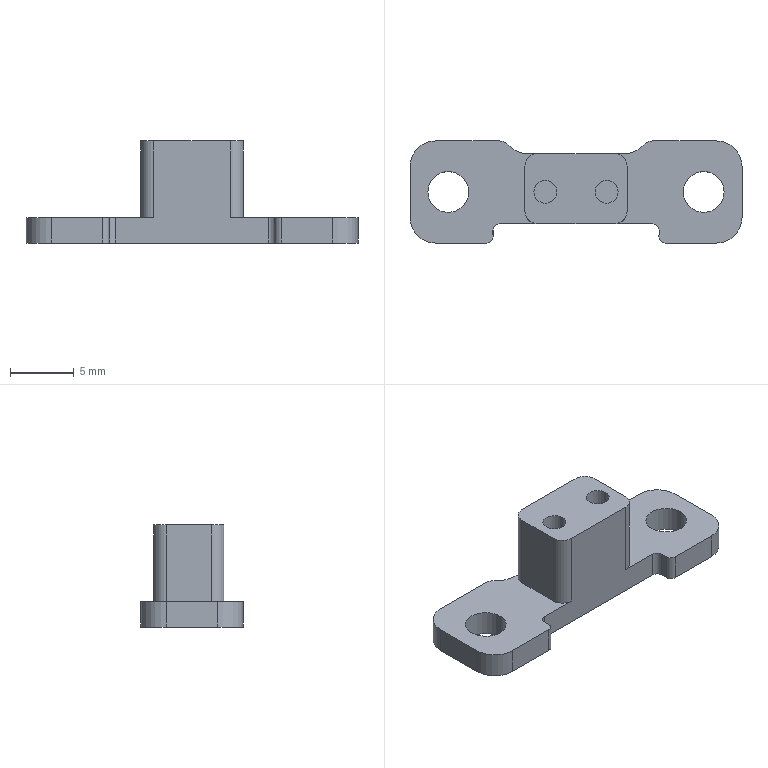NC program | Mastercam | posted with a generic post
Lines 28 to 1213 of 12913:
(8 FEM |TOOL - 8|DIA. OFF. - 8|LEN. - 8|TOOL DIA. - 8.)
N134 T8 M6
N136 G0 G54 G90 X-18.469 Y-15.865 C0. B0. S7000 M3
N138 G43 H8 Z50.
N140 Z-6.696
N142 G1 Z-7.196 F600.
N144 X-18.67 Y-15.925 Z-7.233 F4000.
N146 X-18.876 Y-15.963 Z-7.27
N148 X-19.085 Y-15.979 Z-7.307
N150 X-19.294 Y-15.973 Z-7.344
N152 X-19.501 Y-15.946 Z-7.381
N154 X-19.705 Y-15.897 Z-7.418
N156 X-19.902 Y-15.827 Z-7.455
N158 X-20.091 Y-15.736 Z-7.491
N160 X-20.269 Y-15.627 Z-7.528
N162 X-20.435 Y-15.499 Z-7.565
N164 X-20.587 Y-15.355 Z-7.602
N166 X-20.723 Y-15.196 Z-7.639
N168 X-20.841 Y-15.023 Z-7.676
N170 X-20.941 Y-14.839 Z-7.713
N172 X-21.021 Y-14.646 Z-7.75
N174 X-21.829 Y-12.359
N176 X-22.16 Y-11.421 Z-7.849
N178 X-22.398 Y-10.746 Z-7.92
N180 X-22.476 Y-10.561 Z-7.94
N182 X-22.573 Y-10.386 Z-7.96
N184 X-22.689 Y-10.222 Z-7.98
N186 X-22.823 Y-10.073 Z-8.
N188 X-23.064 Y-9.697
N190 X-23.25 Y-9.308
N192 X-23.4 Y-8.939
N194 X-23.521 Y-8.596
N196 X-23.614 Y-8.279
N198 X-23.685 Y-7.988
N200 X-23.738 Y-7.719
N202 X-23.777 Y-7.471
N204 X-23.83 Y-7.036
N206 X-23.862 Y-6.643
N208 X-23.882 Y-6.282
N210 X-23.893 Y-5.944
N212 X-23.9 Y-5.621
N214 X-23.904 Y-5.309
N216 X-23.906 Y-5.005
N218 X-23.907 Y-4.706
N220 Y-4.41
N222 X-23.906 Y-4.117
N224 X-23.905 Y-3.825
N226 X-23.904 Y-3.535
N228 X-23.903 Y-3.244
N230 X-23.901 Y-2.954
N232 X-23.9 Y-2.664
N234 X-23.898 Y-2.374
N236 X-23.897 Y-2.084
N238 X-23.895 Y-1.794
N240 X-23.894 Y-1.504
N242 X-23.892 Y-1.214
N244 X-23.891 Y-.924
N246 X-23.889 Y-.634
N248 X-23.887 Y-.344
N250 X-23.886 Y-.053
N252 X-23.884 Y.237
N254 X-23.883 Y.527
N256 X-23.881 Y.817
N258 X-23.88 Y1.108
N260 X-23.878 Y1.398
N262 X-23.877 Y1.688
N264 X-23.875 Y1.979
N266 X-23.874 Y2.269
N268 X-23.872 Y2.56
N270 X-23.871 Y2.85
N272 X-23.869 Y3.141
N274 X-23.867 Y3.432
N276 X-23.866 Y3.722
N278 X-23.864 Y4.013
N280 X-23.863 Y4.304
N282 X-23.861 Y4.595
N284 X-23.86 Y4.885
N286 X-23.858 Y5.176
N288 X-23.857 Y5.467
N290 X-23.855 Y5.758
N292 X-23.854 Y6.049
N294 X-23.852 Y6.34
N296 X-23.851 Y6.631
N298 X-23.832 Y7.022
N300 X-23.763 Y7.461
N302 X-23.646 Y7.891
N304 X-23.483 Y8.306
N306 X-23.28 Y8.696
N308 X-23.046 Y9.056
N310 X-22.786 Y9.384
N312 X-22.508 Y9.678
N314 X-22.22 Y9.938
N316 X-21.926 Y10.165
N318 X-21.631 Y10.362
N320 X-21.34 Y10.531
N322 X-21.054 Y10.677
N324 X-20.776 Y10.801
N326 X-20.507 Y10.906
N328 X-20.246 Y10.996
N330 X-19.995 Y11.072
N332 X-19.754 Y11.137
N334 X-19.521 Y11.191
N336 X-19.09 Y11.276
N338 X-18.683 Y11.339
N340 X-18.298 Y11.386
N342 X-17.931 Y11.421
N344 X-17.579 Y11.447
N346 X-17.239 Y11.466
N348 X-16.909 Y11.481
N350 X-16.588 Y11.492
N352 X-16.272 Y11.5
N354 X-15.962 Y11.505
N356 X-15.655 Y11.509
N358 X-15.352 Y11.512
N360 X-15.051 Y11.513
N362 X-14.753 Y11.514
N364 X-14.456
N366 X-14.16
N368 X-13.865
N370 X-13.571 Y11.513
N372 X-13.278 Y11.512
N374 X-12.985 Y11.51
N376 X-12.692 Y11.509
N378 X-12.399 Y11.508
N380 X-12.106 Y11.506
N382 X-11.814 Y11.505
N384 X-11.521 Y11.504
N386 X-11.229 Y11.502
N388 X-10.936 Y11.501
N390 X-10.644 Y11.499
N392 X-10.352 Y11.497
N394 X-10.059 Y11.496
N396 X-9.767 Y11.494
N398 X-9.475 Y11.493
N400 X-9.182 Y11.491
N402 X-8.89 Y11.49
N404 X-8.597 Y11.488
N406 X-8.305 Y11.487
N408 X-8.012 Y11.485
N410 X-7.72 Y11.484
N412 X-7.428 Y11.482
N414 X-7.135 Y11.48
N416 X-6.843 Y11.479
N418 X-6.55 Y11.477
N420 X-6.258 Y11.476
N422 X-5.965 Y11.474
N424 X-5.672 Y11.473
N426 X-5.38 Y11.471
N428 X-5.087 Y11.47
N430 X-4.795 Y11.468
N432 X-4.502 Y11.467
N434 X-4.21 Y11.465
N436 X-3.917 Y11.463
N438 X-3.624 Y11.462
N440 X-3.332 Y11.46
N442 X-3.039 Y11.459
N444 X-2.747 Y11.457
N446 X-2.454 Y11.456
N448 X-2.161 Y11.454
N450 X-1.869 Y11.453
N452 X-1.576 Y11.451
N454 X-1.283 Y11.449
N456 X-.99 Y11.448
N458 X-.698 Y11.446
N460 X-.405 Y11.445
N462 X-.112 Y11.443
N464 X.181 Y11.442
N466 X.473 Y11.44
N468 X.766 Y11.439
N470 X1.059 Y11.437
N472 X1.352 Y11.435
N474 X1.645 Y11.434
N476 X1.937 Y11.432
N478 X2.23 Y11.431
N480 X2.523 Y11.429
N482 X2.816 Y11.428
N484 X3.109 Y11.426
N486 X3.402 Y11.425
N488 X3.694 Y11.423
N490 X3.987 Y11.422
N492 X4.28 Y11.42
N494 X4.573 Y11.418
N496 X4.866 Y11.417
N498 X5.159 Y11.415
N500 X5.452 Y11.414
N502 X5.745 Y11.412
N504 X6.038 Y11.411
N506 X6.331 Y11.409
N508 X6.624 Y11.408
N510 X6.917 Y11.406
N512 X7.21 Y11.404
N514 X7.503 Y11.403
N516 X7.796 Y11.401
N518 X8.089 Y11.4
N520 X8.382 Y11.398
N522 X8.675 Y11.397
N524 X8.968 Y11.395
N526 X9.261 Y11.394
N528 X9.554 Y11.392
N530 X9.847 Y11.39
N532 X10.14 Y11.389
N534 X10.433 Y11.387
N536 X10.726 Y11.386
N538 X11.019 Y11.384
N540 X11.312 Y11.383
N542 X11.606 Y11.381
N544 X11.899 Y11.38
N546 X12.192 Y11.378
N548 X12.485 Y11.376
N550 X12.778 Y11.375
N552 X13.071 Y11.373
N554 X13.364 Y11.372
N556 X13.658 Y11.37
N558 X13.951 Y11.369
N560 X14.244 Y11.367
N562 X14.537 Y11.366
N564 X14.83 Y11.364
N566 X15.124 Y11.362
N568 X15.417 Y11.361
N570 X15.71 Y11.359
N572 X16.004 Y11.358
N574 X16.298 Y11.357
N576 X16.592 Y11.356
N578 X16.887 Y11.355
N580 X17.182 Y11.354
N582 X17.477 Y11.353
N584 X17.773
N586 X18.068 Y11.352
N588 X18.462 Y11.347
N590 X18.756 Y11.318
N592 X19.054 Y11.266
N594 X19.354 Y11.189
N596 X19.651 Y11.089
N598 X19.942 Y10.965
N600 X20.225 Y10.821
N602 X20.497 Y10.658
N604 X20.756 Y10.477
N606 X21. Y10.283
N608 X21.229 Y10.077
N610 X21.442 Y9.861
N612 X21.64 Y9.637
N614 X21.822 Y9.409
N616 X21.988 Y9.177
N618 X22.141 Y8.943
N620 X22.279 Y8.709
N622 X22.405 Y8.475
N624 X22.519 Y8.243
N626 X22.623 Y8.013
N628 X22.716 Y7.785
N630 X22.8 Y7.561
N632 X22.876 Y7.34
N634 X23.004 Y6.917
N636 X23.109 Y6.507
N638 X23.194 Y6.11
N640 X23.264 Y5.726
N642 X23.322 Y5.353
N644 X23.369 Y4.99
N646 X23.408 Y4.637
N648 X23.44 Y4.291
N650 X23.466 Y3.953
N652 X23.488 Y3.621
N654 X23.506 Y3.294
N656 X23.522 Y2.972
N658 X23.534 Y2.653
N660 X23.545 Y2.338
N662 X23.554 Y2.026
N664 X23.561 Y1.716
N666 X23.567 Y1.408
N668 X23.572 Y1.102
N670 X23.577 Y.798
N672 X23.58 Y.494
N674 X23.584 Y.192
N676 X23.586 Y-.109
N678 X23.588 Y-.41
N680 X23.59 Y-.71
N682 X23.592 Y-1.009
N684 X23.593 Y-1.308
N686 X23.594 Y-1.607
N688 X23.595 Y-1.905
N690 X23.596 Y-2.203
N692 Y-2.501
N694 X23.597 Y-2.798
N696 Y-3.095
N698 X23.598 Y-3.393
N700 Y-3.69
N702 Y-3.987
N704 X23.599 Y-4.284
N706 Y-4.581
N708 Y-4.877
N710 Y-5.174
N712 Y-5.471
N714 X23.592 Y-5.741
N716 X23.561 Y-6.036
N718 X23.506 Y-6.335
N720 X23.427 Y-6.634
N722 X23.324 Y-6.931
N724 X23.199 Y-7.222
N726 X23.052 Y-7.503
N728 X22.887 Y-7.774
N730 X22.705 Y-8.031
N732 X22.51 Y-8.274
N734 X22.302 Y-8.501
N736 X22.085 Y-8.713
N738 X21.862 Y-8.909
N740 X21.633 Y-9.089
N742 X21.4 Y-9.254
N744 X21.167 Y-9.405
N746 X20.932 Y-9.543
N748 X20.699 Y-9.667
N750 X20.466 Y-9.78
N752 X20.237 Y-9.883
N754 X20.009 Y-9.975
N756 X19.786 Y-10.058
N758 X19.565 Y-10.133
N760 X19.143 Y-10.26
N762 X18.734 Y-10.364
N764 X18.337 Y-10.448
N766 X17.954 Y-10.518
N768 X17.581 Y-10.574
N770 X17.219 Y-10.621
N772 X16.866 Y-10.659
N774 X16.521 Y-10.691
N776 X16.183 Y-10.717
N778 X15.851 Y-10.739
N780 X15.524 Y-10.757
N782 X15.202 Y-10.772
N784 X14.884 Y-10.785
N786 X14.569 Y-10.795
N788 X14.257 Y-10.804
N790 X13.947 Y-10.811
N792 X13.64 Y-10.818
N794 X13.334 Y-10.823
N796 X13.029 Y-10.827
N798 X12.726 Y-10.831
N800 X12.424 Y-10.834
N802 X12.122 Y-10.836
N804 X11.822 Y-10.838
N806 X11.522 Y-10.84
N808 X11.223 Y-10.842
N810 X10.924 Y-10.843
N812 X10.625 Y-10.844
N814 X10.327 Y-10.845
N816 X10.029 Y-10.846
N818 X9.731 Y-10.847
N820 X9.434
N822 X9.136 Y-10.848
N824 X8.839
N826 X8.542
N828 X8.245 Y-10.849
N830 X7.948
N832 X7.651
N834 X7.354
N836 X7.058
N838 X6.761
N840 X6.464
N842 X6.168 Y-10.85
N844 X5.871
N846 X5.574
N848 X5.278
N850 X4.981
N852 X4.685
N854 X4.388
N856 X4.092
N858 X3.795
N860 X3.499
N862 X3.202
N864 X2.906
N866 X2.609
N868 X2.313
N870 X2.016
N872 X1.72
N874 X1.423
N876 X1.127
N878 X.83
N880 X.534
N882 X.237
N884 X-.059
N886 X-.356
N888 X-.652
N890 X-.949
N892 X-1.245
N894 X-1.542
N896 X-1.838
N898 X-2.135
N900 X-2.431
N902 X-2.728
N904 X-3.024
N906 X-3.321
N908 X-3.617
N910 X-3.914
N912 X-4.21
N914 X-4.507
N916 X-4.803
N918 X-5.1
N920 X-5.396
N922 X-5.693
N924 X-5.989
N926 X-6.286
N928 X-6.582
N930 X-6.879
N932 X-7.175
N934 X-7.472
N936 X-7.768
N938 X-8.065
N940 X-8.361
N942 X-8.657
N944 X-8.954
N946 X-9.25
N948 X-9.547
N950 X-9.843
N952 X-10.14
N954 X-10.436
N956 X-10.733
N958 X-11.029
N960 X-11.326
N962 X-11.622
N964 X-11.919
N966 X-12.215
N968 X-12.512
N970 X-12.808
N972 X-13.105
N974 X-13.401
N976 X-13.698
N978 X-13.994
N980 X-14.291
N982 X-14.587
N984 X-14.884
N986 X-15.18
N988 X-15.477
N990 X-15.773
N992 X-16.07
N994 X-16.366
N996 X-16.663
N998 X-16.959
N1000 X-17.255
N1002 X-17.552
N1004 X-17.848
N1006 X-18.281 Y-10.841
N1008 X-18.592 Y-10.808
N1010 X-18.9 Y-10.752
N1012 X-19.205 Y-10.672
N1014 X-19.506 Y-10.57
N1016 X-19.798 Y-10.447
N1018 X-20.081 Y-10.303
N1020 X-20.353 Y-10.142
N1022 X-20.611 Y-9.965
N1024 X-20.856 Y-9.773
N1026 X-21.086 Y-9.57
N1028 X-21.301 Y-9.357
N1030 X-21.501 Y-9.137
N1032 X-21.685 Y-8.91
N1034 X-21.855 Y-8.68
N1036 X-22.01 Y-8.447
N1038 X-22.152 Y-8.214
N1040 X-22.281 Y-7.98
N1042 X-22.398 Y-7.747
N1044 X-22.504 Y-7.516
N1046 X-22.6 Y-7.288
N1048 X-22.686 Y-7.062
N1050 X-22.764 Y-6.84
N1052 X-22.835 Y-6.621
N1054 X-22.953 Y-6.202
N1056 X-23.05 Y-5.795
N1058 X-23.129 Y-5.402
N1060 X-23.193 Y-5.02
N1062 X-23.246 Y-4.65
N1064 X-23.288 Y-4.29
N1066 X-23.323 Y-3.938
N1068 X-23.352 Y-3.595
N1070 X-23.375 Y-3.258
N1072 X-23.395 Y-2.927
N1074 X-23.41 Y-2.601
N1076 X-23.423 Y-2.28
N1078 X-23.433 Y-1.963
N1080 X-23.442 Y-1.648
N1082 X-23.448 Y-1.337
N1084 X-23.454 Y-1.027
N1086 X-23.458 Y-.72
N1088 X-23.462 Y-.415
N1090 X-23.464 Y-.11
N1092 X-23.466 Y.193
N1094 X-23.467 Y.495
N1096 X-23.468 Y.796
N1098 X-23.469 Y1.096
N1100 Y1.396
N1102 Y1.695
N1104 X-23.468 Y1.994
N1106 Y2.293
N1108 X-23.467 Y2.591
N1110 X-23.466 Y2.889
N1112 X-23.465 Y3.186
N1114 X-23.464 Y3.484
N1116 X-23.463 Y3.781
N1118 X-23.462 Y4.078
N1120 X-23.461 Y4.375
N1122 X-23.459 Y4.672
N1124 X-23.457 Y5.025
N1126 X-23.443 Y5.31
N1128 X-23.414 Y5.609
N1130 X-23.367 Y5.912
N1132 X-23.302 Y6.214
N1134 X-23.218 Y6.512
N1136 X-23.117 Y6.804
N1138 X-22.998 Y7.089
N1140 X-22.863 Y7.366
N1142 X-22.713 Y7.633
N1144 X-22.548 Y7.889
N1146 X-22.372 Y8.133
N1148 X-22.185 Y8.364
N1150 X-21.988 Y8.582
N1152 X-21.783 Y8.787
N1154 X-21.573 Y8.979
N1156 X-21.356 Y9.159
N1158 X-21.137 Y9.326
N1160 X-20.914 Y9.48
N1162 X-20.69 Y9.623
N1164 X-20.464 Y9.755
N1166 X-20.24 Y9.875
N1168 X-20.015 Y9.986
N1170 X-19.792 Y10.087
N1172 X-19.57 Y10.18
N1174 X-19.352 Y10.264
N1176 X-19.134 Y10.342
N1178 X-18.717 Y10.474
N1180 X-18.31 Y10.583
N1182 X-17.913 Y10.674
N1184 X-17.527 Y10.749
N1186 X-17.151 Y10.812
N1188 X-16.785 Y10.863
N1190 X-16.427 Y10.905
N1192 X-16.077 Y10.94
N1194 X-15.735 Y10.969
N1196 X-15.398 Y10.993
N1198 X-15.068 Y11.012
N1200 X-14.742 Y11.028
N1202 X-14.421 Y11.042
N1204 X-14.103 Y11.052
N1206 X-13.788 Y11.061
N1208 X-13.476 Y11.068
N1210 X-13.167 Y11.074
N1212 X-12.859 Y11.078
N1214 X-12.553 Y11.082
N1216 X-12.249 Y11.084
N1218 X-11.946 Y11.087
N1220 X-11.643 Y11.088
N1222 X-11.342 Y11.089
N1224 X-11.042 Y11.09
N1226 X-10.742
N1228 X-10.442
N1230 X-10.143 Y11.089
N1232 X-9.845
N1234 X-9.547 Y11.088
N1236 X-9.249
N1238 X-8.951 Y11.087
N1240 X-8.653 Y11.086
N1242 X-8.356 Y11.084
N1244 X-8.059 Y11.083
N1246 X-7.762 Y11.082
N1248 X-7.465 Y11.081
N1250 X-7.168 Y11.079
N1252 X-6.871 Y11.078
N1254 X-6.574 Y11.077
N1256 X-6.277 Y11.075
N1258 X-5.981 Y11.074
N1260 X-5.684 Y11.072
N1262 X-5.387 Y11.071
N1264 X-5.091 Y11.069
N1266 X-4.794 Y11.068
N1268 X-4.497 Y11.066
N1270 X-4.201 Y11.065
N1272 X-3.904 Y11.063
N1274 X-3.608 Y11.062
N1276 X-3.311 Y11.06
N1278 X-3.015 Y11.059
N1280 X-2.718 Y11.057
N1282 X-2.422 Y11.055
N1284 X-2.125 Y11.054
N1286 X-1.829 Y11.052
N1288 X-1.532 Y11.051
N1290 X-1.236 Y11.049
N1292 X-.939 Y11.048
N1294 X-.643 Y11.046
N1296 X-.346 Y11.044
N1298 X-.05 Y11.043
N1300 X.247 Y11.041
N1302 X.543 Y11.04
N1304 X.84 Y11.038
N1306 X1.136 Y11.037
N1308 X1.433 Y11.035
N1310 X1.729 Y11.033
N1312 X2.026 Y11.032
N1314 X2.322 Y11.03
N1316 X2.619 Y11.029
N1318 X2.915 Y11.027
N1320 X3.212 Y11.026
N1322 X3.508 Y11.024
N1324 X3.805 Y11.022
N1326 X4.101 Y11.021
N1328 X4.397 Y11.019
N1330 X4.694 Y11.018
N1332 X4.99 Y11.016
N1334 X5.287 Y11.015
N1336 X5.583 Y11.013
N1338 X5.88 Y11.011
N1340 X6.176 Y11.01
N1342 X6.473 Y11.008
N1344 X6.769 Y11.007
N1346 X7.066 Y11.005
N1348 X7.362 Y11.004
N1350 X7.659 Y11.002
N1352 X7.955 Y11.
N1354 X8.252 Y10.999
N1356 X8.548 Y10.997
N1358 X8.845 Y10.996
N1360 X9.141 Y10.994
N1362 X9.438 Y10.993
N1364 X9.734 Y10.991
N1366 X10.031 Y10.989
N1368 X10.327 Y10.988
N1370 X10.624 Y10.986
N1372 X10.92 Y10.985
N1374 X11.216 Y10.983
N1376 X11.513 Y10.982
N1378 X11.809 Y10.98
N1380 X12.106 Y10.978
N1382 X12.402 Y10.977
N1384 X12.699 Y10.975
N1386 X12.995 Y10.974
N1388 X13.292 Y10.972
N1390 X13.588 Y10.971
N1392 X13.885 Y10.969
N1394 X14.181 Y10.967
N1396 X14.477 Y10.966
N1398 X14.773 Y10.964
N1400 X15.068 Y10.963
N1402 X15.364 Y10.962
N1404 X15.659 Y10.96
N1406 X15.955 Y10.959
N1408 X16.25 Y10.958
N1410 X16.586 Y10.957
N1412 X16.86 Y10.946
N1414 X17.149 Y10.922
N1416 X17.442 Y10.883
N1418 X17.736 Y10.827
N1420 X18.028 Y10.755
N1422 X18.316 Y10.667
N1424 X18.598 Y10.563
N1426 X18.872 Y10.445
N1428 X19.139 Y10.313
N1430 X19.397 Y10.168
N1432 X19.646 Y10.01
N1434 X19.883 Y9.842
N1436 X20.109 Y9.665
N1438 X20.324 Y9.48
N1440 X20.527 Y9.287
N1442 X20.719 Y9.089
N1444 X20.901 Y8.885
N1446 X21.07 Y8.678
N1448 X21.23 Y8.466
N1450 X21.378 Y8.254
N1452 X21.517 Y8.039
N1454 X21.645 Y7.824
N1456 X21.765 Y7.608
N1458 X21.876 Y7.394
N1460 X21.979 Y7.178
N1462 X22.074 Y6.966
N1464 X22.162 Y6.753
N1466 X22.316 Y6.342
N1468 X22.447 Y5.939
N1470 X22.558 Y5.543
N1472 X22.653 Y5.156
N1474 X22.734 Y4.777
N1476 X22.803 Y4.406
N1478 X22.861 Y4.043
N1480 X22.911 Y3.687
N1482 X22.953 Y3.338
N1484 X22.989 Y2.995
N1486 X23.02 Y2.657
N1488 X23.046 Y2.325
N1490 X23.068 Y1.997
N1492 X23.087 Y1.673
N1494 X23.103 Y1.352
N1496 X23.117 Y1.035
N1498 X23.129 Y.72
N1500 X23.139 Y.408
N1502 X23.148 Y.098
N1504 X23.156 Y-.211
N1506 X23.162 Y-.517
N1508 X23.167 Y-.823
N1510 X23.172 Y-1.127
N1512 X23.176 Y-1.43
N1514 X23.179 Y-1.732
N1516 X23.182 Y-2.034
N1518 X23.185 Y-2.334
N1520 X23.187 Y-2.634
N1522 X23.189 Y-2.934
N1524 X23.191 Y-3.233
N1526 X23.192 Y-3.532
N1528 X23.191 Y-3.914
N1530 X23.177 Y-4.197
N1532 X23.149 Y-4.489
N1534 X23.105 Y-4.784
N1536 X23.044 Y-5.078
N1538 X22.967 Y-5.369
N1540 X22.875 Y-5.656
N1542 X22.766 Y-5.936
N1544 X22.644 Y-6.209
N1546 X22.507 Y-6.473
N1548 X22.358 Y-6.728
N1550 X22.197 Y-6.974
N1552 X22.026 Y-7.207
N1554 X21.846 Y-7.431
N1556 X21.659 Y-7.641
N1558 X21.463 Y-7.842
N1560 X21.263 Y-8.03
N1562 X21.057 Y-8.208
N1564 X20.849 Y-8.374
N1566 X20.637 Y-8.53
N1568 X20.424 Y-8.675
N1570 X20.208 Y-8.811
N1572 X19.993 Y-8.937
N1574 X19.777 Y-9.054
N1576 X19.562 Y-9.162
N1578 X19.348 Y-9.262
N1580 X19.135 Y-9.355
N1582 X18.722 Y-9.517
N1584 X18.316 Y-9.655
N1586 X17.917 Y-9.773
N1588 X17.527 Y-9.873
N1590 X17.145 Y-9.959
N1592 X16.771 Y-10.031
N1594 X16.405 Y-10.093
N1596 X16.047 Y-10.145
N1598 X15.696 Y-10.19
N1600 X15.351 Y-10.228
N1602 X15.011 Y-10.26
N1604 X14.677 Y-10.288
N1606 X14.348 Y-10.311
N1608 X14.023 Y-10.331
N1610 X13.701 Y-10.348
N1612 X13.383 Y-10.363
N1614 X13.067 Y-10.376
N1616 X12.754 Y-10.386
N1618 X12.443 Y-10.395
N1620 X12.134 Y-10.403
N1622 X11.827 Y-10.41
N1624 X11.521 Y-10.416
N1626 X11.217 Y-10.421
N1628 X10.913 Y-10.425
N1630 X10.611 Y-10.428
N1632 X10.309 Y-10.432
N1634 X10.008 Y-10.434
N1636 X9.708 Y-10.436
N1638 X9.408 Y-10.438
N1640 X9.109 Y-10.44
N1642 X8.81 Y-10.442
N1644 X8.511 Y-10.443
N1646 X8.213 Y-10.444
N1648 X7.915 Y-10.445
N1650 X7.617
N1652 X7.319 Y-10.446
N1654 X7.022 Y-10.447
N1656 X6.725
N1658 X6.427 Y-10.448
N1660 X6.13
N1662 X5.833
N1664 X5.536
N1666 X5.239 Y-10.449
N1668 X4.943
N1670 X4.646
N1672 X4.349
N1674 X4.052
N1676 X3.756
N1678 X3.459
N1680 X3.163 Y-10.45
N1682 X2.866
N1684 X2.569
N1686 X2.273
N1688 X1.976
N1690 X1.68
N1692 X1.383
N1694 X1.087
N1696 X.79
N1698 X.494
N1700 X.197
N1702 X-.099
N1704 X-.396
N1706 X-.692
N1708 X-.989
N1710 X-1.285
N1712 X-1.582
N1714 X-1.878
N1716 X-2.175
N1718 X-2.471
N1720 X-2.768
N1722 X-3.064
N1724 X-3.361
N1726 X-3.657
N1728 X-3.954
N1730 X-4.25
N1732 X-4.547
N1734 X-4.843
N1736 X-5.14
N1738 X-5.436
N1740 X-5.733
N1742 X-6.029
N1744 X-6.326
N1746 X-6.622
N1748 X-6.919
N1750 X-7.215
N1752 X-7.512
N1754 X-7.808
N1756 X-8.105
N1758 X-8.401
N1760 X-8.698
N1762 X-8.994
N1764 X-9.291
N1766 X-9.587
N1768 X-9.884
N1770 X-10.18
N1772 X-10.477
N1774 X-10.773
N1776 X-11.069
N1778 X-11.366
N1780 X-11.662
N1782 X-11.959
N1784 X-12.255
N1786 X-12.552
N1788 X-12.848
N1790 X-13.145
N1792 X-13.441
N1794 X-13.738
N1796 X-14.034
N1798 X-14.331
N1800 X-14.627
N1802 X-14.924
N1804 X-15.22
N1806 X-15.517
N1808 X-15.813
N1810 X-16.111
N1812 X-16.482 Y-10.447
N1814 X-16.751 Y-10.435
N1816 X-17.035 Y-10.41
N1818 X-17.324 Y-10.37
N1820 X-17.616 Y-10.315
N1822 X-17.905 Y-10.243
N1824 X-18.191 Y-10.156
N1826 X-18.472 Y-10.053
N1828 X-18.746 Y-9.936
N1830 X-19.012 Y-9.806
N1832 X-19.269 Y-9.662
N1834 X-19.517 Y-9.507
N1836 X-19.756 Y-9.34
N1838 X-19.983 Y-9.164
N1840 X-20.198 Y-8.98
N1842 X-20.403 Y-8.788
N1844 X-20.596 Y-8.59
N1846 X-20.778 Y-8.388
N1848 X-20.949 Y-8.18
N1850 X-21.109 Y-7.971
N1852 X-21.259 Y-7.757
N1854 X-21.399 Y-7.544
N1856 X-21.529 Y-7.328
N1858 X-21.65 Y-7.113
N1860 X-21.762 Y-6.896
N1862 X-21.866 Y-6.682
N1864 X-21.962 Y-6.468
N1866 X-22.051 Y-6.256
N1868 X-22.206 Y-5.844
N1870 X-22.338 Y-5.439
N1872 X-22.451 Y-5.041
N1874 X-22.547 Y-4.652
N1876 X-22.628 Y-4.271
N1878 X-22.697 Y-3.899
N1880 X-22.755 Y-3.534
N1882 X-22.804 Y-3.177
N1884 X-22.846 Y-2.826
N1886 X-22.881 Y-2.482
N1888 X-22.911 Y-2.144
N1890 X-22.936 Y-1.81
N1892 X-22.957 Y-1.481
N1894 X-22.975 Y-1.156
N1896 X-22.99 Y-.835
N1898 X-23.003 Y-.517
N1900 X-23.013 Y-.202
N1902 X-23.022 Y.111
N1904 X-23.03 Y.422
N1906 X-23.036 Y.73
N1908 X-23.041 Y1.037
N1910 X-23.045 Y1.343
N1912 X-23.048 Y1.648
N1914 X-23.051 Y1.951
N1916 X-23.052 Y2.253
N1918 X-23.054 Y2.555
N1920 X-23.055 Y2.856
N1922 X-23.056 Y3.158
N1924 X-23.054 Y3.503
N1926 X-23.039 Y3.942
N1928 X-23.019 Y4.194
N1930 X-22.989 Y4.459
N1932 X-22.947 Y4.731
N1934 X-22.891 Y5.006
N1936 X-22.823 Y5.281
N1938 X-22.74 Y5.555
N1940 X-22.644 Y5.827
N1942 X-22.536 Y6.093
N1944 X-22.414 Y6.353
N1946 X-22.281 Y6.607
N1948 X-22.136 Y6.853
N1950 X-21.981 Y7.09
N1952 X-21.817 Y7.318
N1954 X-21.643 Y7.538
N1956 X-21.463 Y7.746
N1958 X-21.275 Y7.945
N1960 X-21.083 Y8.132
N1962 X-20.884 Y8.312
N1964 X-20.683 Y8.48
N1966 X-20.477 Y8.639
N1968 X-20.27 Y8.787
N1970 X-20.059 Y8.928
N1972 X-19.849 Y9.058
N1974 X-19.637 Y9.18
N1976 X-19.425 Y9.294
N1978 X-19.214 Y9.4
N1980 X-19.003 Y9.499
N1982 X-18.793 Y9.591
N1984 X-18.384 Y9.752
N1986 X-17.981 Y9.891
N1988 X-17.585 Y10.01
N1990 X-17.196 Y10.112
N1992 X-16.814 Y10.199
N1994 X-16.44 Y10.274
N1996 X-16.073 Y10.337
N1998 X-15.714 Y10.391
N2000 X-15.361 Y10.437
N2002 X-15.014 Y10.476
N2004 X-14.673 Y10.51
N2006 X-14.337 Y10.538
N2008 X-14.006 Y10.562
N2010 X-13.679 Y10.582
N2012 X-13.355 Y10.599
N2014 X-13.035 Y10.614
N2016 X-12.718 Y10.626
N2018 X-12.404 Y10.636
N2020 X-12.092 Y10.645
N2022 X-11.782 Y10.652
N2024 X-11.473 Y10.658
N2026 X-11.166 Y10.663
N2028 X-10.861 Y10.667
N2030 X-10.557 Y10.67
N2032 X-10.254 Y10.672
N2034 X-9.951 Y10.674
N2036 X-9.65 Y10.676
N2038 X-9.349 Y10.677
N2040 X-9.049
N2042 X-8.749 Y10.678
N2044 X-8.45
N2046 X-8.151 Y10.677
N2048 X-7.853
N2050 X-7.554
N2052 X-7.256 Y10.676
N2054 X-6.959 Y10.675
N2056 X-6.661 Y10.674
N2058 X-6.364 Y10.673
N2060 X-6.066 Y10.672
N2062 X-5.769 Y10.671
N2064 X-5.472 Y10.67
N2066 X-5.175 Y10.668
N2068 X-4.878 Y10.667
N2070 X-4.581 Y10.666
N2072 X-4.284 Y10.664
N2074 X-3.988 Y10.663
N2076 X-3.691 Y10.661
N2078 X-3.394 Y10.66
N2080 X-3.097 Y10.658
N2082 X-2.801 Y10.657
N2084 X-2.504 Y10.655
N2086 X-2.208 Y10.654
N2088 X-1.911 Y10.652
N2090 X-1.615 Y10.651
N2092 X-1.318 Y10.649
N2094 X-1.021 Y10.648
N2096 X-.725 Y10.646
N2098 X-.428 Y10.645
N2100 X-.132 Y10.643
N2102 X.165 Y10.642
N2104 X.461 Y10.64
N2106 X.758 Y10.639
N2108 X1.054 Y10.637
N2110 X1.351 Y10.635
N2112 X1.647 Y10.634
N2114 X1.944 Y10.632
N2116 X2.24 Y10.631
N2118 X2.537 Y10.629
N2120 X2.833 Y10.628
N2122 X3.13 Y10.626
N2124 X3.426 Y10.624
N2126 X3.723 Y10.623
N2128 X4.019 Y10.621
N2130 X4.316 Y10.62
N2132 X4.612 Y10.618
N2134 X4.909 Y10.617
N2136 X5.205 Y10.615
N2138 X5.502 Y10.613
N2140 X5.798 Y10.612
N2142 X6.094 Y10.61
N2144 X6.391 Y10.609
N2146 X6.687 Y10.607
N2148 X6.984 Y10.606
N2150 X7.28 Y10.604
N2152 X7.577 Y10.602
N2154 X7.873 Y10.601
N2156 X8.17 Y10.599
N2158 X8.466 Y10.598
N2160 X8.763 Y10.596
N2162 X9.059 Y10.595
N2164 X9.356 Y10.593
N2166 X9.652 Y10.591
N2168 X9.949 Y10.59
N2170 X10.245 Y10.588
N2172 X10.542 Y10.587
N2174 X10.838 Y10.585
N2176 X11.135 Y10.584
N2178 X11.431 Y10.582
N2180 X11.728 Y10.58
N2182 X12.024 Y10.579
N2184 X12.321 Y10.577
N2186 X12.617 Y10.576
N2188 X12.913 Y10.574
N2190 X13.21 Y10.573
N2192 X13.506 Y10.571
N2194 X13.802 Y10.57
N2196 X14.098 Y10.568
N2198 X14.394 Y10.567
N2200 X14.69 Y10.565
N2202 X15.006 Y10.563
N2204 X15.394 Y10.554
N2206 X15.618 Y10.543
N2208 X15.856 Y10.525
N2210 X16.106 Y10.497
N2212 X16.364 Y10.46
N2214 X16.626 Y10.412
N2216 X16.891 Y10.352
N2218 X17.156 Y10.28
N2220 X17.42 Y10.197
N2222 X17.681 Y10.102
N2224 X17.938 Y9.994
N2226 X18.19 Y9.876
N2228 X18.436 Y9.747
N2230 X18.675 Y9.608
N2232 X18.907 Y9.46
N2234 X19.131 Y9.303
N2236 X19.347 Y9.137
N2238 X19.554 Y8.964
N2240 X19.752 Y8.786
N2242 X19.94 Y8.602
N2244 X20.12 Y8.412
N2246 X20.29 Y8.22
N2248 X20.453 Y8.022
N2250 X20.605 Y7.823
N2252 X20.75 Y7.621
N2254 X20.886 Y7.418
N2256 X21.015 Y7.212
N2258 X21.135 Y7.007
N2260 X21.248 Y6.8
N2262 X21.354 Y6.595
N2264 X21.453 Y6.389
N2266 X21.63 Y5.987
N2268 X21.784 Y5.589
N2270 X21.919 Y5.196
N2272 X22.036 Y4.808
N2274 X22.138 Y4.427
N2276 X22.226 Y4.052
N2278 X22.303 Y3.683
N2280 X22.369 Y3.321
N2282 X22.426 Y2.964
N2284 X22.476 Y2.614
N2286 X22.519 Y2.269
N2288 X22.557 Y1.928
N2290 X22.589 Y1.593
N2292 X22.617 Y1.262
N2294 X22.641 Y.934
N2296 X22.662 Y.61
N2298 X22.681 Y.289
N2300 X22.697 Y-.029
N2302 X22.71 Y-.344
N2304 X22.722 Y-.657
N2306 X22.733 Y-.969
N2308 X22.742 Y-1.278
N2310 X22.749 Y-1.586
N2312 X22.756 Y-1.894
N2314 X22.761 Y-2.226
N2316 X22.759 Y-2.632
N2318 X22.75 Y-2.864
N2320 X22.733 Y-3.109
N2322 X22.707 Y-3.365
N2324 X22.671 Y-3.627
N2326 X22.623 Y-3.893
N2328 X22.563 Y-4.161
N2330 X22.491 Y-4.429
N2332 X22.407 Y-4.695
N2334 X22.311 Y-4.957
N2336 X22.203 Y-5.216
N2338 X22.084 Y-5.469
N2340 X21.954 Y-5.716
N2342 X21.814 Y-5.955
N2344 X21.664 Y-6.187
N2346 X21.505 Y-6.412
N2348 X21.338 Y-6.628
N2350 X21.165 Y-6.833
N2352 X20.985 Y-7.031
N2354 X20.8 Y-7.219
N2356 X20.61 Y-7.398
N2358 X20.416 Y-7.568
N2360 X20.219 Y-7.728
N2362 X20.018 Y-7.881
N2364 X19.816 Y-8.024
N2366 X19.611 Y-8.16
N2368 X19.407 Y-8.286
N2370 X19.199 Y-8.406
N2372 X18.994 Y-8.518
N2374 X18.787 Y-8.623
N2376 X18.384 Y-8.81
N2378 X17.984 Y-8.974
N2380 X17.588 Y-9.116
N2382 X17.198 Y-9.241
N2384 X16.814 Y-9.348
N2386 X16.436 Y-9.442
N2388 X16.064 Y-9.523
N2390 X15.699 Y-9.594
N2392 X15.341 Y-9.655
N2394 X14.988 Y-9.707
N2396 X14.64 Y-9.753
N2398 X14.298 Y-9.793
N2400 X13.961 Y-9.827
N2402 X13.628 Y-9.857
N2404 X13.299 Y-9.882
N2406 X12.973 Y-9.905
N2408 X12.651 Y-9.924
N2410 X12.332 Y-9.941
N2412 X12.016 Y-9.955
N2414 X11.702 Y-9.968
N2416 X11.39 Y-9.979
N2418 X11.08 Y-9.988
N2420 X10.771 Y-9.996
N2422 X10.464 Y-10.004
N2424 X10.159 Y-10.01
N2426 X9.854 Y-10.015
N2428 X9.551 Y-10.02
N2430 X9.248 Y-10.024
N2432 X8.946 Y-10.027
N2434 X8.645 Y-10.03
N2436 X8.344 Y-10.033
N2438 X8.044 Y-10.035
N2440 X7.745 Y-10.037
N2442 X7.445 Y-10.039
N2444 X7.147 Y-10.041
N2446 X6.848 Y-10.042
N2448 X6.55 Y-10.043
N2450 X6.252 Y-10.044
N2452 X5.954 Y-10.045
N2454 X5.656
N2456 X5.359 Y-10.046
N2458 X5.061 Y-10.047
N2460 X4.764
N2462 X4.467
N2464 X4.17 Y-10.048
N2466 X3.873
N2468 X3.576
N2470 X3.279 Y-10.049
N2472 X2.982
N2474 X2.686
N2476 X2.389
N2478 X2.092
N2480 X1.796
N2482 X1.499
N2484 X1.202
N2486 X.906 Y-10.05
N2488 X.609
N2490 X.313
N2492 X.016
N2494 X-.28
N2496 X-.577
N2498 X-.874
N2500 X-1.17
N2502 X-1.467